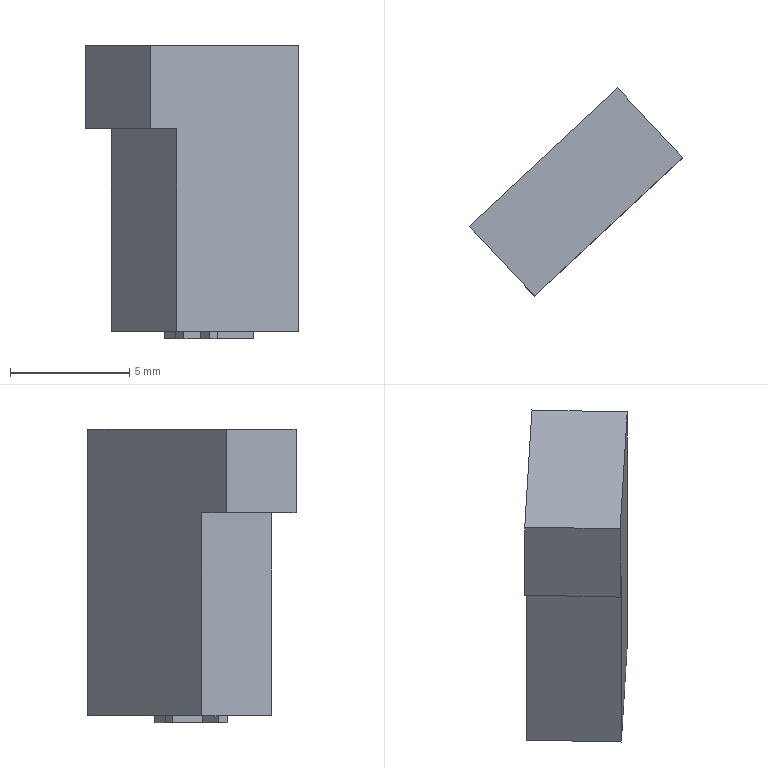Part | STEP file | gslz 2016.10.28-13_id858_x_t | 1 solid | 24 faces | box 8.945 x 8.722 x 12.3 mm | volume 358.198 mm3 | plane 24